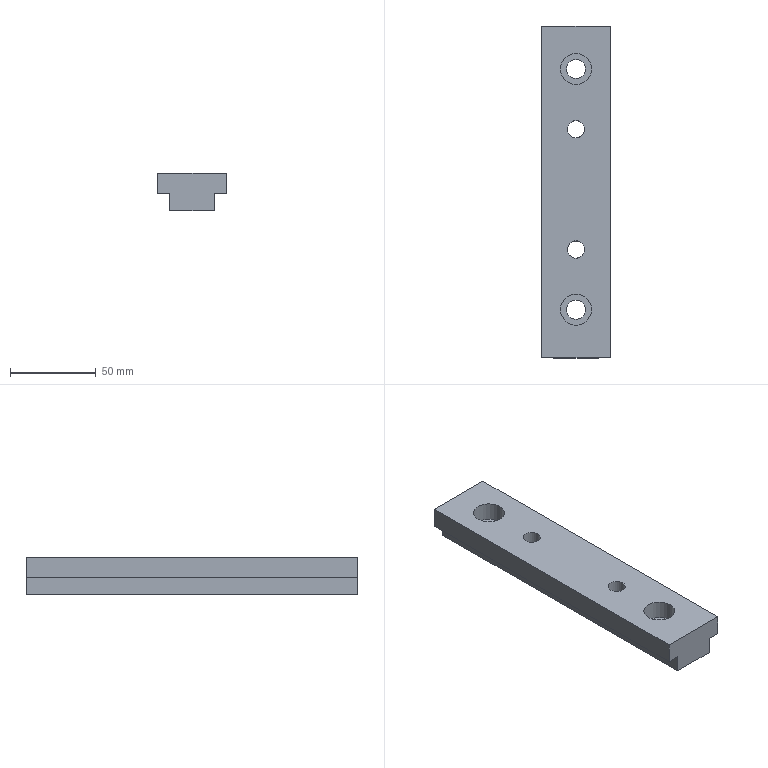Part | STEP file | solid 96 | 1 solid | 18 faces | box 40 x 193.057 x 22 mm | volume 131718 mm3 | plane 12 | cylinder 6 | commonest cylinder face diameters 10 x2 11 x2 18 x2